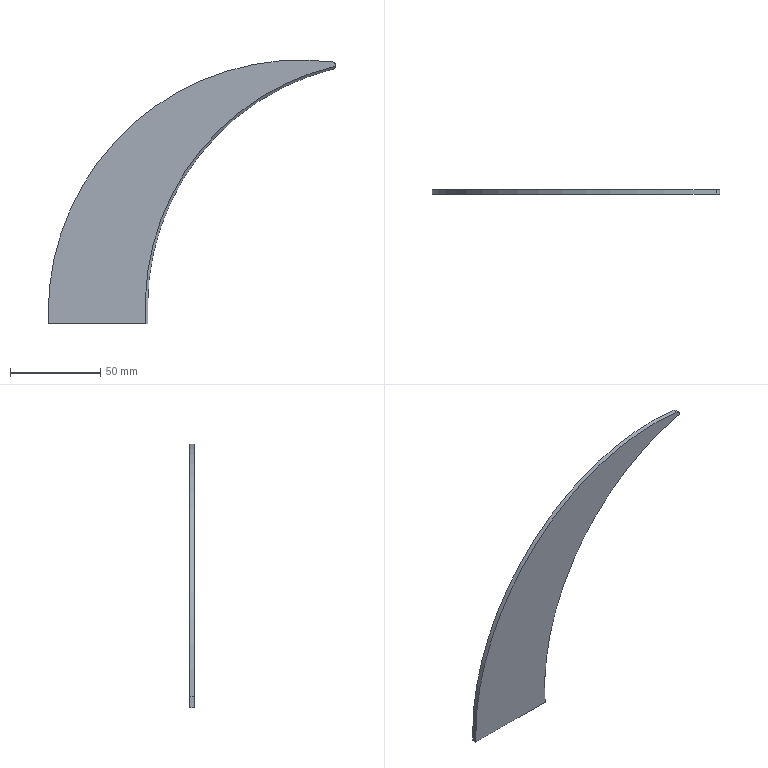Part | STEP file | DEWALT-DWE7492-B22 | 1 solid | 9 faces | box 159.2 x 2.5 x 146.092 mm | volume 19224 mm3 | plane 5 | cylinder 2 | cone 2 | commonest cylinder face diameters 4 x1 280 x1
STEP:
#1=CARTESIAN_POINT('',(0.,0.,0.));
#2=DIRECTION('',(0.,0.,1.));
#3=DIRECTION('',(1.,0.,0.));
#4=AXIS2_PLACEMENT_3D('',#1,#2,#3);
#5=CARTESIAN_POINT('',(54.117,2.5,0.));
#6=VERTEX_POINT('',#5);
#7=CARTESIAN_POINT('',(0.,2.5,0.));
#8=VERTEX_POINT('',#7);
#9=CARTESIAN_POINT('',(55.,2.5,0.));
#10=DIRECTION('',(-1.,0.,0.));
#11=VECTOR('',#10,1.);
#12=LINE('',#9,#11);
#13=CARTESIAN_POINT('',(55.,2.5,0.));
#14=DIRECTION('',(0.,0.,1.));
#15=DIRECTION('',(1.,0.,0.));
#16=AXIS2_PLACEMENT_3D('',#13,#14,#15);
#17=PLANE('',#16);
#18=CARTESIAN_POINT('',(0.,0.));
#19=DIRECTION('',(-1.,0.));
#20=VECTOR('',#19,1.);
#21=LINE('',#18,#20);
#22=(GEOMETRIC_REPRESENTATION_CONTEXT(2)PARAMETRIC_REPRESENTATION_CONTEXT()REPRESENTATION_CONTEXT('',''));
#23=DEFINITIONAL_REPRESENTATION('',(#21),#22);
#24=PCURVE('',#17,#23);
#25=CARTESIAN_POINT('',(140.,2.5,6.092));
#26=DIRECTION('',(0.,1.,0.));
#27=DIRECTION('',(0.,0.,1.));
#28=AXIS2_PLACEMENT_3D('',#25,#26,#27);
#29=PLANE('',#28);
#30=CARTESIAN_POINT('',(-6.092,-85.));
#31=DIRECTION('',(0.,-1.));
#32=VECTOR('',#31,1.);
#33=LINE('',#30,#32);
#34=(GEOMETRIC_REPRESENTATION_CONTEXT(2)PARAMETRIC_REPRESENTATION_CONTEXT()REPRESENTATION_CONTEXT('',''));
#35=DEFINITIONAL_REPRESENTATION('',(#33),#34);
#36=PCURVE('',#29,#35);
#37=SURFACE_CURVE('',#12,(#24,#36),.PCURVE_S1.);
#38=EDGE_CURVE('',#6,#8,#37,.T.);
#39=ORIENTED_EDGE('',*,*,#38,.F.);
#40=CARTESIAN_POINT('',(55.,1.62,0.));
#41=VERTEX_POINT('',#40);
#42=CARTESIAN_POINT('',(54.117,2.5,0.));
#43=CARTESIAN_POINT('',(54.412,2.207,0.));
#44=CARTESIAN_POINT('',(54.706,1.913,0.));
#45=CARTESIAN_POINT('',(55.,1.62,0.));
#46=B_SPLINE_CURVE_WITH_KNOTS('',3,(#42,#43,#44,#45),.UNSPECIFIED.,.F.,.F.,(4,4),(0.,0.001246),.PIECEWISE_BEZIER_KNOTS.);
#47=CARTESIAN_POINT('',(-0.8825,0.));
#48=CARTESIAN_POINT('',(-0.5884,-0.2934));
#49=CARTESIAN_POINT('',(-0.2942,-0.5868));
#50=CARTESIAN_POINT('',(0.,-0.8801));
#51=B_SPLINE_CURVE_WITH_KNOTS('',3,(#47,#48,#49,#50),.UNSPECIFIED.,.F.,.F.,(4,4),(0.,0.001246),.PIECEWISE_BEZIER_KNOTS.);
#52=(GEOMETRIC_REPRESENTATION_CONTEXT(2)PARAMETRIC_REPRESENTATION_CONTEXT()REPRESENTATION_CONTEXT('',''));
#53=DEFINITIONAL_REPRESENTATION('',(#51),#52);
#54=PCURVE('',#17,#53);
#55=CARTESIAN_POINT('',(190.,2.5,10.));
#56=DIRECTION('',(0.,1.,0.));
#57=DIRECTION('',(0.,0.,1.));
#58=AXIS2_PLACEMENT_3D('',#55,#56,#57);
#59=CONICAL_SURFACE('',#58,136.25,0.7854);
#60=CARTESIAN_POINT('',(4.639,0.));
#61=CARTESIAN_POINT('',(4.638,-0.8801));
#62=B_SPLINE_CURVE_WITH_KNOTS('',1,(#60,#61),.UNSPECIFIED.,.F.,.F.,(2,2),(0.,0.001246),.PIECEWISE_BEZIER_KNOTS.);
#63=(GEOMETRIC_REPRESENTATION_CONTEXT(2)PARAMETRIC_REPRESENTATION_CONTEXT()REPRESENTATION_CONTEXT('',''));
#64=DEFINITIONAL_REPRESENTATION('',(#62),#63);
#65=PCURVE('',#59,#64);
#66=SURFACE_CURVE('',#46,(#54,#65),.PCURVE_S1.);
#67=EDGE_CURVE('',#6,#41,#66,.T.);
#68=ORIENTED_EDGE('',*,*,#67,.T.);
#69=CARTESIAN_POINT('',(55.,0.8801,0.));
#70=VERTEX_POINT('',#69);
#71=CARTESIAN_POINT('',(55.,2.5,0.));
#72=DIRECTION('',(0.,-1.,0.));
#73=VECTOR('',#72,1.);
#74=LINE('',#71,#73);
#75=CARTESIAN_POINT('',(0.,0.));
#76=DIRECTION('',(0.,-1.));
#77=VECTOR('',#76,1.);
#78=LINE('',#75,#77);
#79=(GEOMETRIC_REPRESENTATION_CONTEXT(2)PARAMETRIC_REPRESENTATION_CONTEXT()REPRESENTATION_CONTEXT('',''));
#80=DEFINITIONAL_REPRESENTATION('',(#78),#79);
#81=PCURVE('',#17,#80);
#82=CARTESIAN_POINT('',(55.,2.5,10.));
#83=DIRECTION('',(-1.,0.,0.));
#84=DIRECTION('',(0.,0.,1.));
#85=AXIS2_PLACEMENT_3D('',#82,#83,#84);
#86=PLANE('',#85);
#87=CARTESIAN_POINT('',(-10.,0.));
#88=DIRECTION('',(0.,-1.));
#89=VECTOR('',#88,1.);
#90=LINE('',#87,#89);
#91=(GEOMETRIC_REPRESENTATION_CONTEXT(2)PARAMETRIC_REPRESENTATION_CONTEXT()REPRESENTATION_CONTEXT('',''));
#92=DEFINITIONAL_REPRESENTATION('',(#90),#91);
#93=PCURVE('',#86,#92);
#94=SURFACE_CURVE('',#74,(#81,#93),.PCURVE_S1.);
#95=EDGE_CURVE('',#41,#70,#94,.T.);
#96=ORIENTED_EDGE('',*,*,#95,.T.);
#97=CARTESIAN_POINT('',(54.117,0.,0.));
#98=VERTEX_POINT('',#97);
#99=CARTESIAN_POINT('',(55.,0.8801,0.));
#100=CARTESIAN_POINT('',(54.706,0.5868,0.));
#101=CARTESIAN_POINT('',(54.412,0.2934,0.));
#102=CARTESIAN_POINT('',(54.117,0.,0.));
#103=B_SPLINE_CURVE_WITH_KNOTS('',3,(#99,#100,#101,#102),.UNSPECIFIED.,.F.,.F.,(4,4),(0.,0.001246),.PIECEWISE_BEZIER_KNOTS.);
#104=CARTESIAN_POINT('',(0.,-1.62));
#105=CARTESIAN_POINT('',(-0.2942,-1.913));
#106=CARTESIAN_POINT('',(-0.5884,-2.207));
#107=CARTESIAN_POINT('',(-0.8825,-2.5));
#108=B_SPLINE_CURVE_WITH_KNOTS('',3,(#104,#105,#106,#107),.UNSPECIFIED.,.F.,.F.,(4,4),(0.,0.001246),.PIECEWISE_BEZIER_KNOTS.);
#109=(GEOMETRIC_REPRESENTATION_CONTEXT(2)PARAMETRIC_REPRESENTATION_CONTEXT()REPRESENTATION_CONTEXT('',''));
#110=DEFINITIONAL_REPRESENTATION('',(#108),#109);
#111=PCURVE('',#17,#110);
#112=CARTESIAN_POINT('',(190.,1.25,10.));
#113=DIRECTION('',(0.,-1.,0.));
#114=DIRECTION('',(0.,0.,-1.));
#115=AXIS2_PLACEMENT_3D('',#112,#113,#114);
#116=CONICAL_SURFACE('',#115,135.,0.7854);
#117=CARTESIAN_POINT('',(4.786,0.3699));
#118=CARTESIAN_POINT('',(4.786,1.25));
#119=B_SPLINE_CURVE_WITH_KNOTS('',1,(#117,#118),.UNSPECIFIED.,.F.,.F.,(2,2),(0.,0.001246),.PIECEWISE_BEZIER_KNOTS.);
#120=(GEOMETRIC_REPRESENTATION_CONTEXT(2)PARAMETRIC_REPRESENTATION_CONTEXT()REPRESENTATION_CONTEXT('',''));
#121=DEFINITIONAL_REPRESENTATION('',(#119),#120);
#122=PCURVE('',#116,#121);
#123=SURFACE_CURVE('',#103,(#111,#122),.PCURVE_S1.);
#124=EDGE_CURVE('',#70,#98,#123,.T.);
#125=ORIENTED_EDGE('',*,*,#124,.T.);
#126=CARTESIAN_POINT('',(0.,0.,0.));
#127=VERTEX_POINT('',#126);
#128=CARTESIAN_POINT('',(55.,0.,0.));
#129=DIRECTION('',(-1.,0.,0.));
#130=VECTOR('',#129,1.);
#131=LINE('',#128,#130);
#132=CARTESIAN_POINT('',(0.,-2.5));
#133=DIRECTION('',(-1.,0.));
#134=VECTOR('',#133,1.);
#135=LINE('',#132,#134);
#136=(GEOMETRIC_REPRESENTATION_CONTEXT(2)PARAMETRIC_REPRESENTATION_CONTEXT()REPRESENTATION_CONTEXT('',''));
#137=DEFINITIONAL_REPRESENTATION('',(#135),#136);
#138=PCURVE('',#17,#137);
#139=CARTESIAN_POINT('',(140.,0.,6.092));
#140=DIRECTION('',(0.,1.,0.));
#141=DIRECTION('',(0.,0.,1.));
#142=AXIS2_PLACEMENT_3D('',#139,#140,#141);
#143=PLANE('',#142);
#144=CARTESIAN_POINT('',(-6.092,-85.));
#145=DIRECTION('',(0.,-1.));
#146=VECTOR('',#145,1.);
#147=LINE('',#144,#146);
#148=(GEOMETRIC_REPRESENTATION_CONTEXT(2)PARAMETRIC_REPRESENTATION_CONTEXT()REPRESENTATION_CONTEXT('',''));
#149=DEFINITIONAL_REPRESENTATION('',(#147),#148);
#150=PCURVE('',#143,#149);
#151=SURFACE_CURVE('',#131,(#138,#150),.PCURVE_S1.);
#152=EDGE_CURVE('',#98,#127,#151,.T.);
#153=ORIENTED_EDGE('',*,*,#152,.T.);
#154=CARTESIAN_POINT('',(0.,2.5,0.));
#155=DIRECTION('',(0.,-1.,0.));
#156=VECTOR('',#155,1.);
#157=LINE('',#154,#156);
#158=CARTESIAN_POINT('',(-55.,0.));
#159=DIRECTION('',(0.,-1.));
#160=VECTOR('',#159,1.);
#161=LINE('',#158,#160);
#162=(GEOMETRIC_REPRESENTATION_CONTEXT(2)PARAMETRIC_REPRESENTATION_CONTEXT()REPRESENTATION_CONTEXT('',''));
#163=DEFINITIONAL_REPRESENTATION('',(#161),#162);
#164=PCURVE('',#17,#163);
#165=CARTESIAN_POINT('',(0.,2.5,0.));
#166=DIRECTION('',(1.,0.,0.));
#167=DIRECTION('',(0.,0.,-1.));
#168=AXIS2_PLACEMENT_3D('',#165,#166,#167);
#169=PLANE('',#168);
#170=CARTESIAN_POINT('',(0.,0.));
#171=DIRECTION('',(0.,-1.));
#172=VECTOR('',#171,1.);
#173=LINE('',#170,#172);
#174=(GEOMETRIC_REPRESENTATION_CONTEXT(2)PARAMETRIC_REPRESENTATION_CONTEXT()REPRESENTATION_CONTEXT('',''));
#175=DEFINITIONAL_REPRESENTATION('',(#173),#174);
#176=PCURVE('',#169,#175);
#177=SURFACE_CURVE('',#157,(#164,#176),.PCURVE_S1.);
#178=EDGE_CURVE('',#8,#127,#177,.T.);
#179=ORIENTED_EDGE('',*,*,#178,.F.);
#180=EDGE_LOOP('',(#39,#68,#96,#125,#153,#179));
#181=FACE_BOUND('',#180,.T.);
#182=ADVANCED_FACE('',(#181),#17,.F.);
#183=CARTESIAN_POINT('',(0.,0.,6.092));
#184=VERTEX_POINT('',#183);
#185=CARTESIAN_POINT('',(0.,0.,0.));
#186=DIRECTION('',(0.,0.,1.));
#187=VECTOR('',#186,1.);
#188=LINE('',#185,#187);
#189=CARTESIAN_POINT('',(0.,-2.5));
#190=DIRECTION('',(-1.,0.));
#191=VECTOR('',#190,1.);
#192=LINE('',#189,#191);
#193=(GEOMETRIC_REPRESENTATION_CONTEXT(2)PARAMETRIC_REPRESENTATION_CONTEXT()REPRESENTATION_CONTEXT('',''));
#194=DEFINITIONAL_REPRESENTATION('',(#192),#193);
#195=PCURVE('',#169,#194);
#196=CARTESIAN_POINT('',(-6.092,-140.));
#197=DIRECTION('',(1.,0.));
#198=VECTOR('',#197,1.);
#199=LINE('',#196,#198);
#200=(GEOMETRIC_REPRESENTATION_CONTEXT(2)PARAMETRIC_REPRESENTATION_CONTEXT()REPRESENTATION_CONTEXT('',''));
#201=DEFINITIONAL_REPRESENTATION('',(#199),#200);
#202=PCURVE('',#143,#201);
#203=SURFACE_CURVE('',#188,(#195,#202),.PCURVE_S1.);
#204=EDGE_CURVE('',#127,#184,#203,.T.);
#205=ORIENTED_EDGE('',*,*,#204,.T.);
#206=CARTESIAN_POINT('',(0.,2.5,6.092));
#207=VERTEX_POINT('',#206);
#208=CARTESIAN_POINT('',(0.,2.5,6.092));
#209=DIRECTION('',(0.,-1.,0.));
#210=VECTOR('',#209,1.);
#211=LINE('',#208,#210);
#212=CARTESIAN_POINT('',(-6.092,0.));
#213=DIRECTION('',(0.,-1.));
#214=VECTOR('',#213,1.);
#215=LINE('',#212,#214);
#216=(GEOMETRIC_REPRESENTATION_CONTEXT(2)PARAMETRIC_REPRESENTATION_CONTEXT()REPRESENTATION_CONTEXT('',''));
#217=DEFINITIONAL_REPRESENTATION('',(#215),#216);
#218=PCURVE('',#169,#217);
#219=CARTESIAN_POINT('',(140.,2.5,6.092));
#220=DIRECTION('',(0.,-1.,0.));
#221=DIRECTION('',(0.,0.,-1.));
#222=AXIS2_PLACEMENT_3D('',#219,#220,#221);
#223=CYLINDRICAL_SURFACE('',#222,140.);
#224=CARTESIAN_POINT('',(4.712,0.));
#225=DIRECTION('',(0.,1.));
#226=VECTOR('',#225,1.);
#227=LINE('',#224,#226);
#228=(GEOMETRIC_REPRESENTATION_CONTEXT(2)PARAMETRIC_REPRESENTATION_CONTEXT()REPRESENTATION_CONTEXT('',''));
#229=DEFINITIONAL_REPRESENTATION('',(#227),#228);
#230=PCURVE('',#223,#229);
#231=SURFACE_CURVE('',#211,(#218,#230),.PCURVE_S1.);
#232=EDGE_CURVE('',#207,#184,#231,.T.);
#233=ORIENTED_EDGE('',*,*,#232,.F.);
#234=CARTESIAN_POINT('',(0.,2.5,0.));
#235=DIRECTION('',(0.,0.,1.));
#236=VECTOR('',#235,1.);
#237=LINE('',#234,#236);
#238=CARTESIAN_POINT('',(0.,0.));
#239=DIRECTION('',(-1.,0.));
#240=VECTOR('',#239,1.);
#241=LINE('',#238,#240);
#242=(GEOMETRIC_REPRESENTATION_CONTEXT(2)PARAMETRIC_REPRESENTATION_CONTEXT()REPRESENTATION_CONTEXT('',''));
#243=DEFINITIONAL_REPRESENTATION('',(#241),#242);
#244=PCURVE('',#169,#243);
#245=CARTESIAN_POINT('',(-6.092,-140.));
#246=DIRECTION('',(1.,0.));
#247=VECTOR('',#246,1.);
#248=LINE('',#245,#247);
#249=(GEOMETRIC_REPRESENTATION_CONTEXT(2)PARAMETRIC_REPRESENTATION_CONTEXT()REPRESENTATION_CONTEXT('',''));
#250=DEFINITIONAL_REPRESENTATION('',(#248),#249);
#251=PCURVE('',#29,#250);
#252=SURFACE_CURVE('',#237,(#244,#251),.PCURVE_S1.);
#253=EDGE_CURVE('',#8,#207,#252,.T.);
#254=ORIENTED_EDGE('',*,*,#253,.F.);
#255=ORIENTED_EDGE('',*,*,#178,.T.);
#256=EDGE_LOOP('',(#205,#233,#254,#255));
#257=FACE_BOUND('',#256,.T.);
#258=ADVANCED_FACE('',(#257),#169,.F.);
#259=CARTESIAN_POINT('',(157.449,0.,145.));
#260=VERTEX_POINT('',#259);
#261=CARTESIAN_POINT('',(140.,0.,6.092));
#262=DIRECTION('',(0.,1.,0.));
#263=DIRECTION('',(1.,0.,0.));
#264=AXIS2_PLACEMENT_3D('',#261,#262,#263);
#265=CIRCLE('',#264,140.);
#266=CARTESIAN_POINT('',(7.854,2.5));
#267=DIRECTION('',(-1.,0.));
#268=VECTOR('',#267,1.);
#269=LINE('',#266,#268);
#270=(GEOMETRIC_REPRESENTATION_CONTEXT(2)PARAMETRIC_REPRESENTATION_CONTEXT()REPRESENTATION_CONTEXT('',''));
#271=DEFINITIONAL_REPRESENTATION('',(#269),#270);
#272=PCURVE('',#223,#271);
#273=CARTESIAN_POINT('',(0.,0.));
#274=DIRECTION('',(0.,1.));
#275=AXIS2_PLACEMENT_2D('',#273,#274);
#276=CIRCLE('',#275,140.);
#277=(GEOMETRIC_REPRESENTATION_CONTEXT(2)PARAMETRIC_REPRESENTATION_CONTEXT()REPRESENTATION_CONTEXT('',''));
#278=DEFINITIONAL_REPRESENTATION('',(#276),#277);
#279=PCURVE('',#143,#278);
#280=SURFACE_CURVE('',#265,(#272,#279),.PCURVE_S1.);
#281=EDGE_CURVE('',#184,#260,#280,.T.);
#282=ORIENTED_EDGE('',*,*,#281,.T.);
#283=CARTESIAN_POINT('',(157.449,2.5,145.));
#284=VERTEX_POINT('',#283);
#285=CARTESIAN_POINT('',(157.449,2.5,145.));
#286=DIRECTION('',(0.,-1.,0.));
#287=VECTOR('',#286,1.);
#288=LINE('',#285,#287);
#289=CARTESIAN_POINT('',(3.017,0.));
#290=DIRECTION('',(0.,1.));
#291=VECTOR('',#290,1.);
#292=LINE('',#289,#291);
#293=(GEOMETRIC_REPRESENTATION_CONTEXT(2)PARAMETRIC_REPRESENTATION_CONTEXT()REPRESENTATION_CONTEXT('',''));
#294=DEFINITIONAL_REPRESENTATION('',(#292),#293);
#295=PCURVE('',#223,#294);
#296=CARTESIAN_POINT('',(157.2,2.5,143.016));
#297=DIRECTION('',(0.,-1.,0.));
#298=DIRECTION('',(0.,0.,-1.));
#299=AXIS2_PLACEMENT_3D('',#296,#297,#298);
#300=CYLINDRICAL_SURFACE('',#299,2.);
#301=CARTESIAN_POINT('',(3.017,0.));
#302=DIRECTION('',(0.,1.));
#303=VECTOR('',#302,1.);
#304=LINE('',#301,#303);
#305=(GEOMETRIC_REPRESENTATION_CONTEXT(2)PARAMETRIC_REPRESENTATION_CONTEXT()REPRESENTATION_CONTEXT('',''));
#306=DEFINITIONAL_REPRESENTATION('',(#304),#305);
#307=PCURVE('',#300,#306);
#308=SURFACE_CURVE('',#288,(#295,#307),.PCURVE_S1.);
#309=EDGE_CURVE('',#284,#260,#308,.T.);
#310=ORIENTED_EDGE('',*,*,#309,.F.);
#311=CARTESIAN_POINT('',(140.,2.5,6.092));
#312=DIRECTION('',(0.,1.,0.));
#313=DIRECTION('',(1.,0.,0.));
#314=AXIS2_PLACEMENT_3D('',#311,#312,#313);
#315=CIRCLE('',#314,140.);
#316=CARTESIAN_POINT('',(7.854,0.));
#317=DIRECTION('',(-1.,0.));
#318=VECTOR('',#317,1.);
#319=LINE('',#316,#318);
#320=(GEOMETRIC_REPRESENTATION_CONTEXT(2)PARAMETRIC_REPRESENTATION_CONTEXT()REPRESENTATION_CONTEXT('',''));
#321=DEFINITIONAL_REPRESENTATION('',(#319),#320);
#322=PCURVE('',#223,#321);
#323=CARTESIAN_POINT('',(0.,0.));
#324=DIRECTION('',(0.,1.));
#325=AXIS2_PLACEMENT_2D('',#323,#324);
#326=CIRCLE('',#325,140.);
#327=(GEOMETRIC_REPRESENTATION_CONTEXT(2)PARAMETRIC_REPRESENTATION_CONTEXT()REPRESENTATION_CONTEXT('',''));
#328=DEFINITIONAL_REPRESENTATION('',(#326),#327);
#329=PCURVE('',#29,#328);
#330=SURFACE_CURVE('',#315,(#322,#329),.PCURVE_S1.);
#331=EDGE_CURVE('',#207,#284,#330,.T.);
#332=ORIENTED_EDGE('',*,*,#331,.F.);
#333=ORIENTED_EDGE('',*,*,#232,.T.);
#334=EDGE_LOOP('',(#282,#310,#332,#333));
#335=FACE_BOUND('',#334,.T.);
#336=ADVANCED_FACE('',(#335),#223,.T.);
#337=CARTESIAN_POINT('',(159.178,0.,142.718));
#338=VERTEX_POINT('',#337);
#339=CARTESIAN_POINT('',(157.679,1.25,141.074));
#340=VERTEX_POINT('',#339);
#341=CARTESIAN_POINT('',(159.178,0.,142.718));
#342=CARTESIAN_POINT('',(159.128,0.3116,142.386));
#343=CARTESIAN_POINT('',(158.872,0.9052,141.718));
#344=CARTESIAN_POINT('',(158.127,1.25,141.184));
#345=CARTESIAN_POINT('',(157.679,1.25,141.074));
#346=B_SPLINE_CURVE_WITH_KNOTS('',3,(#341,#342,#343,#344,#345),.UNSPECIFIED.,.F.,.F.,(4,1,4),(0.,0.001357,0.002714),.UNSPECIFIED.);
#347=CARTESIAN_POINT('',(1.421,2.5));
#348=CARTESIAN_POINT('',(1.406,2.472));
#349=CARTESIAN_POINT('',(1.376,2.415));
#350=CARTESIAN_POINT('',(1.329,2.332));
#351=CARTESIAN_POINT('',(1.283,2.249));
#352=CARTESIAN_POINT('',(1.236,2.168));
#353=CARTESIAN_POINT('',(1.188,2.088));
#354=CARTESIAN_POINT('',(1.14,2.011));
#355=CARTESIAN_POINT('',(1.091,1.935));
#356=CARTESIAN_POINT('',(1.041,1.861));
#357=CARTESIAN_POINT('',(0.991,1.79));
#358=CARTESIAN_POINT('',(0.9395,1.722));
#359=CARTESIAN_POINT('',(0.8869,1.656));
#360=CARTESIAN_POINT('',(0.8329,1.594));
#361=CARTESIAN_POINT('',(0.7777,1.535));
#362=CARTESIAN_POINT('',(0.7214,1.48));
#363=CARTESIAN_POINT('',(0.6641,1.43));
#364=CARTESIAN_POINT('',(0.606,1.385));
#365=CARTESIAN_POINT('',(0.5471,1.346));
#366=CARTESIAN_POINT('',(0.4875,1.312));
#367=CARTESIAN_POINT('',(0.4271,1.285));
#368=CARTESIAN_POINT('',(0.3661,1.265));
#369=CARTESIAN_POINT('',(0.3044,1.253));
#370=CARTESIAN_POINT('',(0.2627,1.25));
#371=CARTESIAN_POINT('',(0.2418,1.25));
#372=B_SPLINE_CURVE_WITH_KNOTS('',3,(#347,#348,#349,#350,#351,#352,#353,#354,#355,#356,#357,#358,#359,#360,#361,#362,#363,#364,#365,#366,#367,#368,#369,#370,#371),.UNSPECIFIED.,.F.,.F.,(4,1,1,1,1,1,1,1,1,1,1,1,1,1,1,1,1,1,1,1,1,1,4),(0.,0.0001234,0.0002467,0.0003701,0.0004934,0.0006168,0.0007401,0.0008635,0.0009868,0.00111,0.001234,0.001357,0.00148,0.001604,0.001727,0.00185,0.001974,0.002097,0.00222,0.002344,0.002467,0.00259,0.002714),.QUASI_UNIFORM_KNOTS.);
#373=(GEOMETRIC_REPRESENTATION_CONTEXT(2)PARAMETRIC_REPRESENTATION_CONTEXT()REPRESENTATION_CONTEXT('',''));
#374=DEFINITIONAL_REPRESENTATION('',(#372),#373);
#375=PCURVE('',#300,#374);
#376=CARTESIAN_POINT('',(3.37,1.25));
#377=CARTESIAN_POINT('',(3.37,1.222));
#378=CARTESIAN_POINT('',(3.37,1.165));
#379=CARTESIAN_POINT('',(3.37,1.082));
#380=CARTESIAN_POINT('',(3.371,0.9991));
#381=CARTESIAN_POINT('',(3.371,0.918));
#382=CARTESIAN_POINT('',(3.371,0.8384));
#383=CARTESIAN_POINT('',(3.372,0.7607));
#384=CARTESIAN_POINT('',(3.372,0.685));
#385=CARTESIAN_POINT('',(3.373,0.6115));
#386=CARTESIAN_POINT('',(3.373,0.5404));
#387=CARTESIAN_POINT('',(3.374,0.472));
#388=CARTESIAN_POINT('',(3.374,0.4065));
#389=CARTESIAN_POINT('',(3.375,0.344));
#390=CARTESIAN_POINT('',(3.376,0.2852));
#391=CARTESIAN_POINT('',(3.377,0.2304));
#392=CARTESIAN_POINT('',(3.377,0.1802));
#393=CARTESIAN_POINT('',(3.378,0.135));
#394=CARTESIAN_POINT('',(3.379,0.09548));
#395=CARTESIAN_POINT('',(3.38,0.06198));
#396=CARTESIAN_POINT('',(3.381,0.03504));
#397=CARTESIAN_POINT('',(3.382,0.01517));
#398=CARTESIAN_POINT('',(3.382,0.002848));
#399=CARTESIAN_POINT('',(3.383,-0.000000049));
#400=CARTESIAN_POINT('',(3.383,0.));
#401=B_SPLINE_CURVE_WITH_KNOTS('',3,(#376,#377,#378,#379,#380,#381,#382,#383,#384,#385,#386,#387,#388,#389,#390,#391,#392,#393,#394,#395,#396,#397,#398,#399,#400),.UNSPECIFIED.,.F.,.F.,(4,1,1,1,1,1,1,1,1,1,1,1,1,1,1,1,1,1,1,1,1,1,4),(0.,0.0001234,0.0002467,0.0003701,0.0004934,0.0006168,0.0007401,0.0008635,0.0009868,0.00111,0.001234,0.001357,0.00148,0.001604,0.001727,0.00185,0.001974,0.002097,0.00222,0.002344,0.002467,0.00259,0.002714),.QUASI_UNIFORM_KNOTS.);
#402=(GEOMETRIC_REPRESENTATION_CONTEXT(2)PARAMETRIC_REPRESENTATION_CONTEXT()REPRESENTATION_CONTEXT('',''));
#403=DEFINITIONAL_REPRESENTATION('',(#401),#402);
#404=PCURVE('',#116,#403);
#405=SURFACE_CURVE('',#346,(#375,#404),.PCURVE_S1.);
#406=EDGE_CURVE('',#338,#340,#405,.T.);
#407=ORIENTED_EDGE('',*,*,#406,.T.);
#408=CARTESIAN_POINT('',(159.178,2.5,142.718));
#409=VERTEX_POINT('',#408);
#410=CARTESIAN_POINT('',(157.679,1.25,141.074));
#411=CARTESIAN_POINT('',(158.127,1.25,141.184));
#412=CARTESIAN_POINT('',(158.871,1.594,141.717));
#413=CARTESIAN_POINT('',(159.128,2.188,142.386));
#414=CARTESIAN_POINT('',(159.178,2.5,142.718));
#415=B_SPLINE_CURVE_WITH_KNOTS('',3,(#410,#411,#412,#413,#414),.UNSPECIFIED.,.F.,.F.,(4,1,4),(0.,0.00136,0.002721),.UNSPECIFIED.);
#416=CARTESIAN_POINT('',(0.2418,1.25));
#417=CARTESIAN_POINT('',(0.2627,1.25));
#418=CARTESIAN_POINT('',(0.3044,1.247));
#419=CARTESIAN_POINT('',(0.3661,1.235));
#420=CARTESIAN_POINT('',(0.4271,1.215));
#421=CARTESIAN_POINT('',(0.4873,1.188));
#422=CARTESIAN_POINT('',(0.5469,1.155));
#423=CARTESIAN_POINT('',(0.6058,1.115));
#424=CARTESIAN_POINT('',(0.6639,1.07));
#425=CARTESIAN_POINT('',(0.7211,1.02));
#426=CARTESIAN_POINT('',(0.7773,0.9653));
#427=CARTESIAN_POINT('',(0.8325,0.9064));
#428=CARTESIAN_POINT('',(0.8865,0.844));
#429=CARTESIAN_POINT('',(0.9391,0.7785));
#430=CARTESIAN_POINT('',(0.9906,0.7101));
#431=CARTESIAN_POINT('',(1.041,0.639));
#432=CARTESIAN_POINT('',(1.091,0.5654));
#433=CARTESIAN_POINT('',(1.14,0.4896));
#434=CARTESIAN_POINT('',(1.188,0.4118));
#435=CARTESIAN_POINT('',(1.235,0.3322));
#436=CARTESIAN_POINT('',(1.283,0.251));
#437=CARTESIAN_POINT('',(1.329,0.1685));
#438=CARTESIAN_POINT('',(1.376,0.08477));
#439=CARTESIAN_POINT('',(1.406,0.02834));
#440=CARTESIAN_POINT('',(1.421,0.));
#441=B_SPLINE_CURVE_WITH_KNOTS('',3,(#416,#417,#418,#419,#420,#421,#422,#423,#424,#425,#426,#427,#428,#429,#430,#431,#432,#433,#434,#435,#436,#437,#438,#439,#440),.UNSPECIFIED.,.F.,.F.,(4,1,1,1,1,1,1,1,1,1,1,1,1,1,1,1,1,1,1,1,1,1,4),(0.,0.0001237,0.0002473,0.000371,0.0004947,0.0006183,0.000742,0.0008657,0.0009893,0.001113,0.001237,0.00136,0.001484,0.001608,0.001731,0.001855,0.001979,0.002102,0.002226,0.00235,0.002473,0.002597,0.002721),.QUASI_UNIFORM_KNOTS.);
#442=(GEOMETRIC_REPRESENTATION_CONTEXT(2)PARAMETRIC_REPRESENTATION_CONTEXT()REPRESENTATION_CONTEXT('',''));
#443=DEFINITIONAL_REPRESENTATION('',(#441),#442);
#444=PCURVE('',#300,#443);
#445=CARTESIAN_POINT('',(6.041,-1.25));
#446=CARTESIAN_POINT('',(6.042,-1.25));
#447=CARTESIAN_POINT('',(6.042,-1.247));
#448=CARTESIAN_POINT('',(6.043,-1.235));
#449=CARTESIAN_POINT('',(6.044,-1.215));
#450=CARTESIAN_POINT('',(6.045,-1.188));
#451=CARTESIAN_POINT('',(6.046,-1.155));
#452=CARTESIAN_POINT('',(6.047,-1.115));
#453=CARTESIAN_POINT('',(6.047,-1.07));
#454=CARTESIAN_POINT('',(6.048,-1.02));
#455=CARTESIAN_POINT('',(6.049,-0.9653));
#456=CARTESIAN_POINT('',(6.05,-0.9064));
#457=CARTESIAN_POINT('',(6.05,-0.844));
#458=CARTESIAN_POINT('',(6.051,-0.7785));
#459=CARTESIAN_POINT('',(6.051,-0.71));
#460=CARTESIAN_POINT('',(6.052,-0.6389));
#461=CARTESIAN_POINT('',(6.053,-0.5654));
#462=CARTESIAN_POINT('',(6.053,-0.4896));
#463=CARTESIAN_POINT('',(6.053,-0.4118));
#464=CARTESIAN_POINT('',(6.054,-0.3322));
#465=CARTESIAN_POINT('',(6.054,-0.251));
#466=CARTESIAN_POINT('',(6.054,-0.1685));
#467=CARTESIAN_POINT('',(6.055,-0.08477));
#468=CARTESIAN_POINT('',(6.055,-0.02834));
#469=CARTESIAN_POINT('',(6.055,0.));
#470=B_SPLINE_CURVE_WITH_KNOTS('',3,(#445,#446,#447,#448,#449,#450,#451,#452,#453,#454,#455,#456,#457,#458,#459,#460,#461,#462,#463,#464,#465,#466,#467,#468,#469),.UNSPECIFIED.,.F.,.F.,(4,1,1,1,1,1,1,1,1,1,1,1,1,1,1,1,1,1,1,1,1,1,4),(0.,0.0001237,0.0002473,0.000371,0.0004947,0.0006183,0.000742,0.0008657,0.0009893,0.001113,0.001237,0.00136,0.001484,0.001608,0.001731,0.001855,0.001979,0.002102,0.002226,0.00235,0.002473,0.002597,0.002721),.QUASI_UNIFORM_KNOTS.);
#471=(GEOMETRIC_REPRESENTATION_CONTEXT(2)PARAMETRIC_REPRESENTATION_CONTEXT()REPRESENTATION_CONTEXT('',''));
#472=DEFINITIONAL_REPRESENTATION('',(#470),#471);
#473=PCURVE('',#59,#472);
#474=SURFACE_CURVE('',#415,(#444,#473),.PCURVE_S1.);
#475=EDGE_CURVE('',#340,#409,#474,.T.);
#476=ORIENTED_EDGE('',*,*,#475,.T.);
#477=CARTESIAN_POINT('',(157.2,2.5,143.016));
#478=DIRECTION('',(0.,1.,0.));
#479=DIRECTION('',(-1.,0.,0.));
#480=AXIS2_PLACEMENT_3D('',#477,#478,#479);
#481=CIRCLE('',#480,2.);
#482=CARTESIAN_POINT('',(4.712,0.));
#483=DIRECTION('',(-1.,0.));
#484=VECTOR('',#483,1.);
#485=LINE('',#482,#484);
#486=(GEOMETRIC_REPRESENTATION_CONTEXT(2)PARAMETRIC_REPRESENTATION_CONTEXT()REPRESENTATION_CONTEXT('',''));
#487=DEFINITIONAL_REPRESENTATION('',(#485),#486);
#488=PCURVE('',#300,#487);
#489=CARTESIAN_POINT('',(136.924,17.2));
#490=DIRECTION('',(0.,-1.));
#491=AXIS2_PLACEMENT_2D('',#489,#490);
#492=CIRCLE('',#491,2.);
#493=(GEOMETRIC_REPRESENTATION_CONTEXT(2)PARAMETRIC_REPRESENTATION_CONTEXT()REPRESENTATION_CONTEXT('',''));
#494=DEFINITIONAL_REPRESENTATION('',(#492),#493);
#495=PCURVE('',#29,#494);
#496=SURFACE_CURVE('',#481,(#488,#495),.PCURVE_S1.);
#497=EDGE_CURVE('',#284,#409,#496,.T.);
#498=ORIENTED_EDGE('',*,*,#497,.F.);
#499=ORIENTED_EDGE('',*,*,#309,.T.);
#500=CARTESIAN_POINT('',(157.2,0.,143.016));
#501=DIRECTION('',(0.,1.,0.));
#502=DIRECTION('',(-1.,0.,0.));
#503=AXIS2_PLACEMENT_3D('',#500,#501,#502);
#504=CIRCLE('',#503,2.);
#505=CARTESIAN_POINT('',(4.712,2.5));
#506=DIRECTION('',(-1.,0.));
#507=VECTOR('',#506,1.);
#508=LINE('',#505,#507);
#509=(GEOMETRIC_REPRESENTATION_CONTEXT(2)PARAMETRIC_REPRESENTATION_CONTEXT()REPRESENTATION_CONTEXT('',''));
#510=DEFINITIONAL_REPRESENTATION('',(#508),#509);
#511=PCURVE('',#300,#510);
#512=CARTESIAN_POINT('',(136.924,17.2));
#513=DIRECTION('',(0.,-1.));
#514=AXIS2_PLACEMENT_2D('',#512,#513);
#515=CIRCLE('',#514,2.);
#516=(GEOMETRIC_REPRESENTATION_CONTEXT(2)PARAMETRIC_REPRESENTATION_CONTEXT()REPRESENTATION_CONTEXT('',''));
#517=DEFINITIONAL_REPRESENTATION('',(#515),#516);
#518=PCURVE('',#143,#517);
#519=SURFACE_CURVE('',#504,(#511,#518),.PCURVE_S1.);
#520=EDGE_CURVE('',#260,#338,#519,.T.);
#521=ORIENTED_EDGE('',*,*,#520,.T.);
#522=EDGE_LOOP('',(#407,#476,#498,#499,#521));
#523=FACE_BOUND('',#522,.T.);
#524=ADVANCED_FACE('',(#523),#300,.T.);
#525=ORIENTED_EDGE('',*,*,#95,.F.);
#526=CARTESIAN_POINT('',(55.,1.25,10.));
#527=VERTEX_POINT('',#526);
#528=CARTESIAN_POINT('',(55.,1.62,0.));
#529=CARTESIAN_POINT('',(55.,1.374,3.329));
#530=CARTESIAN_POINT('',(55.,1.25,6.662));
#531=CARTESIAN_POINT('',(55.,1.25,10.));
#532=B_SPLINE_CURVE_WITH_KNOTS('',3,(#528,#529,#530,#531),.UNSPECIFIED.,.F.,.F.,(4,4),(0.,0.01001),.PIECEWISE_BEZIER_KNOTS.);
#533=CARTESIAN_POINT('',(-10.,-0.8801));
#534=CARTESIAN_POINT('',(-6.671,-1.126));
#535=CARTESIAN_POINT('',(-3.338,-1.25));
#536=CARTESIAN_POINT('',(0.,-1.25));
#537=B_SPLINE_CURVE_WITH_KNOTS('',3,(#533,#534,#535,#536),.UNSPECIFIED.,.F.,.F.,(4,4),(0.,0.01001),.PIECEWISE_BEZIER_KNOTS.);
#538=(GEOMETRIC_REPRESENTATION_CONTEXT(2)PARAMETRIC_REPRESENTATION_CONTEXT()REPRESENTATION_CONTEXT('',''));
#539=DEFINITIONAL_REPRESENTATION('',(#537),#538);
#540=PCURVE('',#86,#539);
#541=CARTESIAN_POINT('',(4.638,-0.8801));
#542=CARTESIAN_POINT('',(4.64,-0.8913));
#543=CARTESIAN_POINT('',(4.642,-0.9132));
#544=CARTESIAN_POINT('',(4.645,-0.9444));
#545=CARTESIAN_POINT('',(4.648,-0.9742));
#546=CARTESIAN_POINT('',(4.652,-1.002));
#547=CARTESIAN_POINT('',(4.655,-1.029));
#548=CARTESIAN_POINT('',(4.659,-1.054));
#549=CARTESIAN_POINT('',(4.662,-1.078));
#550=CARTESIAN_POINT('',(4.665,-1.1));
#551=CARTESIAN_POINT('',(4.669,-1.121));
#552=CARTESIAN_POINT('',(4.672,-1.14));
#553=CARTESIAN_POINT('',(4.675,-1.158));
#554=CARTESIAN_POINT('',(4.679,-1.174));
#555=CARTESIAN_POINT('',(4.682,-1.188));
#556=CARTESIAN_POINT('',(4.685,-1.201));
#557=CARTESIAN_POINT('',(4.689,-1.213));
#558=CARTESIAN_POINT('',(4.692,-1.223));
#559=CARTESIAN_POINT('',(4.696,-1.231));
#560=CARTESIAN_POINT('',(4.699,-1.238));
#561=CARTESIAN_POINT('',(4.702,-1.243));
#562=CARTESIAN_POINT('',(4.706,-1.247));
#563=CARTESIAN_POINT('',(4.709,-1.249));
#564=CARTESIAN_POINT('',(4.711,-1.25));
#565=CARTESIAN_POINT('',(4.712,-1.25));
#566=B_SPLINE_CURVE_WITH_KNOTS('',3,(#541,#542,#543,#544,#545,#546,#547,#548,#549,#550,#551,#552,#553,#554,#555,#556,#557,#558,#559,#560,#561,#562,#563,#564,#565),.UNSPECIFIED.,.F.,.F.,(4,1,1,1,1,1,1,1,1,1,1,1,1,1,1,1,1,1,1,1,1,1,4),(0.,0.0004549,0.0009097,0.001365,0.001819,0.002274,0.002729,0.003184,0.003639,0.004094,0.004549,0.005003,0.005458,0.005913,0.006368,0.006823,0.007278,0.007733,0.008187,0.008642,0.009097,0.009552,0.01001),.QUASI_UNIFORM_KNOTS.);
#567=(GEOMETRIC_REPRESENTATION_CONTEXT(2)PARAMETRIC_REPRESENTATION_CONTEXT()REPRESENTATION_CONTEXT('',''));
#568=DEFINITIONAL_REPRESENTATION('',(#566),#567);
#569=PCURVE('',#59,#568);
#570=SURFACE_CURVE('',#532,(#540,#569),.PCURVE_S1.);
#571=EDGE_CURVE('',#41,#527,#570,.T.);
#572=ORIENTED_EDGE('',*,*,#571,.T.);
#573=CARTESIAN_POINT('',(55.,1.25,10.));
#574=CARTESIAN_POINT('',(55.,1.25,6.662));
#575=CARTESIAN_POINT('',(55.,1.126,3.329));
#576=CARTESIAN_POINT('',(55.,0.8801,0.));
#577=B_SPLINE_CURVE_WITH_KNOTS('',3,(#573,#574,#575,#576),.UNSPECIFIED.,.F.,.F.,(4,4),(0.,0.01001),.PIECEWISE_BEZIER_KNOTS.);
#578=CARTESIAN_POINT('',(0.,-1.25));
#579=CARTESIAN_POINT('',(-3.338,-1.25));
#580=CARTESIAN_POINT('',(-6.671,-1.374));
#581=CARTESIAN_POINT('',(-10.,-1.62));
#582=B_SPLINE_CURVE_WITH_KNOTS('',3,(#578,#579,#580,#581),.UNSPECIFIED.,.F.,.F.,(4,4),(0.,0.01001),.PIECEWISE_BEZIER_KNOTS.);
#583=(GEOMETRIC_REPRESENTATION_CONTEXT(2)PARAMETRIC_REPRESENTATION_CONTEXT()REPRESENTATION_CONTEXT('',''));
#584=DEFINITIONAL_REPRESENTATION('',(#582),#583);
#585=PCURVE('',#86,#584);
#586=CARTESIAN_POINT('',(4.712,0.));
#587=CARTESIAN_POINT('',(4.714,-0.000000002));
#588=CARTESIAN_POINT('',(4.716,0.0005119));
#589=CARTESIAN_POINT('',(4.719,0.002815));
#590=CARTESIAN_POINT('',(4.723,0.006651));
#591=CARTESIAN_POINT('',(4.726,0.01202));
#592=CARTESIAN_POINT('',(4.729,0.01892));
#593=CARTESIAN_POINT('',(4.733,0.02735));
#594=CARTESIAN_POINT('',(4.736,0.03732));
#595=CARTESIAN_POINT('',(4.739,0.04881));
#596=CARTESIAN_POINT('',(4.743,0.06183));
#597=CARTESIAN_POINT('',(4.746,0.07638));
#598=CARTESIAN_POINT('',(4.749,0.09245));
#599=CARTESIAN_POINT('',(4.753,0.11));
#600=CARTESIAN_POINT('',(4.756,0.1292));
#601=CARTESIAN_POINT('',(4.76,0.1498));
#602=CARTESIAN_POINT('',(4.763,0.172));
#603=CARTESIAN_POINT('',(4.766,0.1957));
#604=CARTESIAN_POINT('',(4.77,0.2209));
#605=CARTESIAN_POINT('',(4.773,0.2476));
#606=CARTESIAN_POINT('',(4.776,0.2758));
#607=CARTESIAN_POINT('',(4.78,0.3056));
#608=CARTESIAN_POINT('',(4.783,0.3368));
#609=CARTESIAN_POINT('',(4.785,0.3587));
#610=CARTESIAN_POINT('',(4.786,0.3699));
#611=B_SPLINE_CURVE_WITH_KNOTS('',3,(#586,#587,#588,#589,#590,#591,#592,#593,#594,#595,#596,#597,#598,#599,#600,#601,#602,#603,#604,#605,#606,#607,#608,#609,#610),.UNSPECIFIED.,.F.,.F.,(4,1,1,1,1,1,1,1,1,1,1,1,1,1,1,1,1,1,1,1,1,1,4),(0.,0.0004549,0.0009097,0.001365,0.001819,0.002274,0.002729,0.003184,0.003639,0.004094,0.004549,0.005003,0.005458,0.005913,0.006368,0.006823,0.007278,0.007733,0.008187,0.008642,0.009097,0.009552,0.01001),.QUASI_UNIFORM_KNOTS.);
#612=(GEOMETRIC_REPRESENTATION_CONTEXT(2)PARAMETRIC_REPRESENTATION_CONTEXT()REPRESENTATION_CONTEXT('',''));
#613=DEFINITIONAL_REPRESENTATION('',(#611),#612);
#614=PCURVE('',#116,#613);
#615=SURFACE_CURVE('',#577,(#585,#614),.PCURVE_S1.);
#616=EDGE_CURVE('',#527,#70,#615,.T.);
#617=ORIENTED_EDGE('',*,*,#616,.T.);
#618=EDGE_LOOP('',(#525,#572,#617));
#619=FACE_BOUND('',#618,.T.);
#620=ADVANCED_FACE('',(#619),#86,.F.);
#621=ORIENTED_EDGE('',*,*,#497,.T.);
#622=CARTESIAN_POINT('',(190.,2.5,10.));
#623=DIRECTION('',(0.,1.,0.));
#624=DIRECTION('',(0.,0.,1.));
#625=AXIS2_PLACEMENT_3D('',#622,#623,#624);
#626=CIRCLE('',#625,136.25);
#627=CARTESIAN_POINT('',(3.908,50.));
#628=DIRECTION('',(1.,0.));
#629=AXIS2_PLACEMENT_2D('',#627,#628);
#630=CIRCLE('',#629,136.25);
#631=(GEOMETRIC_REPRESENTATION_CONTEXT(2)PARAMETRIC_REPRESENTATION_CONTEXT()REPRESENTATION_CONTEXT('',''));
#632=DEFINITIONAL_REPRESENTATION('',(#630),#631);
#633=PCURVE('',#29,#632);
#634=CARTESIAN_POINT('',(0.,0.));
#635=DIRECTION('',(1.,0.));
#636=VECTOR('',#635,1.);
#637=LINE('',#634,#636);
#638=(GEOMETRIC_REPRESENTATION_CONTEXT(2)PARAMETRIC_REPRESENTATION_CONTEXT()REPRESENTATION_CONTEXT('',''));
#639=DEFINITIONAL_REPRESENTATION('',(#637),#638);
#640=PCURVE('',#59,#639);
#641=SURFACE_CURVE('',#626,(#633,#640),.PCURVE_S1.);
#642=EDGE_CURVE('',#6,#409,#641,.T.);
#643=ORIENTED_EDGE('',*,*,#642,.F.);
#644=ORIENTED_EDGE('',*,*,#38,.T.);
#645=ORIENTED_EDGE('',*,*,#253,.T.);
#646=ORIENTED_EDGE('',*,*,#331,.T.);
#647=EDGE_LOOP('',(#621,#643,#644,#645,#646));
#648=FACE_BOUND('',#647,.T.);
#649=ADVANCED_FACE('',(#648),#29,.T.);
#650=ORIENTED_EDGE('',*,*,#152,.F.);
#651=CARTESIAN_POINT('',(190.,0.,10.));
#652=DIRECTION('',(0.,1.,0.));
#653=DIRECTION('',(0.,0.,1.));
#654=AXIS2_PLACEMENT_3D('',#651,#652,#653);
#655=CIRCLE('',#654,136.25);
#656=CARTESIAN_POINT('',(3.908,50.));
#657=DIRECTION('',(1.,0.));
#658=AXIS2_PLACEMENT_2D('',#656,#657);
#659=CIRCLE('',#658,136.25);
#660=(GEOMETRIC_REPRESENTATION_CONTEXT(2)PARAMETRIC_REPRESENTATION_CONTEXT()REPRESENTATION_CONTEXT('',''));
#661=DEFINITIONAL_REPRESENTATION('',(#659),#660);
#662=PCURVE('',#143,#661);
#663=CARTESIAN_POINT('',(9.425,1.25));
#664=DIRECTION('',(-1.,0.));
#665=VECTOR('',#664,1.);
#666=LINE('',#663,#665);
#667=(GEOMETRIC_REPRESENTATION_CONTEXT(2)PARAMETRIC_REPRESENTATION_CONTEXT()REPRESENTATION_CONTEXT('',''));
#668=DEFINITIONAL_REPRESENTATION('',(#666),#667);
#669=PCURVE('',#116,#668);
#670=SURFACE_CURVE('',#655,(#662,#669),.PCURVE_S1.);
#671=EDGE_CURVE('',#98,#338,#670,.T.);
#672=ORIENTED_EDGE('',*,*,#671,.T.);
#673=ORIENTED_EDGE('',*,*,#520,.F.);
#674=ORIENTED_EDGE('',*,*,#281,.F.);
#675=ORIENTED_EDGE('',*,*,#204,.F.);
#676=EDGE_LOOP('',(#650,#672,#673,#674,#675));
#677=FACE_BOUND('',#676,.T.);
#678=ADVANCED_FACE('',(#677),#143,.F.);
#679=CARTESIAN_POINT('',(190.,1.25,10.));
#680=DIRECTION('',(0.,1.,0.));
#681=DIRECTION('',(0.,0.,1.));
#682=AXIS2_PLACEMENT_3D('',#679,#680,#681);
#683=CIRCLE('',#682,135.);
#684=CARTESIAN_POINT('',(9.425,0.));
#685=DIRECTION('',(-1.,0.));
#686=VECTOR('',#685,1.);
#687=LINE('',#684,#686);
#688=(GEOMETRIC_REPRESENTATION_CONTEXT(2)PARAMETRIC_REPRESENTATION_CONTEXT()REPRESENTATION_CONTEXT('',''));
#689=DEFINITIONAL_REPRESENTATION('',(#687),#688);
#690=PCURVE('',#116,#689);
#691=CARTESIAN_POINT('',(0.,-1.25));
#692=DIRECTION('',(1.,0.));
#693=VECTOR('',#692,1.);
#694=LINE('',#691,#693);
#695=(GEOMETRIC_REPRESENTATION_CONTEXT(2)PARAMETRIC_REPRESENTATION_CONTEXT()REPRESENTATION_CONTEXT('',''));
#696=DEFINITIONAL_REPRESENTATION('',(#694),#695);
#697=PCURVE('',#59,#696);
#698=SURFACE_CURVE('',#683,(#690,#697),.PCURVE_S1.);
#699=EDGE_CURVE('',#527,#340,#698,.T.);
#700=ORIENTED_EDGE('',*,*,#699,.F.);
#701=ORIENTED_EDGE('',*,*,#616,.T.);
#702=ORIENTED_EDGE('',*,*,#124,.T.);
#703=ORIENTED_EDGE('',*,*,#671,.T.);
#704=ORIENTED_EDGE('',*,*,#406,.T.);
#705=EDGE_LOOP('',(#700,#701,#702,#703,#704));
#706=FACE_BOUND('',#705,.F.);
#707=ADVANCED_FACE('',(#706),#116,.F.);
#708=ORIENTED_EDGE('',*,*,#642,.F.);
#709=ORIENTED_EDGE('',*,*,#67,.T.);
#710=ORIENTED_EDGE('',*,*,#571,.T.);
#711=ORIENTED_EDGE('',*,*,#699,.T.);
#712=ORIENTED_EDGE('',*,*,#475,.T.);
#713=EDGE_LOOP('',(#708,#709,#710,#711,#712));
#714=FACE_BOUND('',#713,.F.);
#715=ADVANCED_FACE('',(#714),#59,.F.);
#716=CLOSED_SHELL('',(#182,#258,#336,#524,#620,#649,#678,#707,#715));
#717=MANIFOLD_SOLID_BREP('',#716);
#718=(LENGTH_UNIT()NAMED_UNIT(*)SI_UNIT(.MILLI.,.METRE.));
#719=UNCERTAINTY_MEASURE_WITH_UNIT(LENGTH_MEASURE(0.0005),#718,'','');
#720=(NAMED_UNIT(*)PLANE_ANGLE_UNIT()SI_UNIT($,.RADIAN.));
#721=(NAMED_UNIT(*)SI_UNIT($,.STERADIAN.)SOLID_ANGLE_UNIT());
#722=(GEOMETRIC_REPRESENTATION_CONTEXT(3)GLOBAL_UNCERTAINTY_ASSIGNED_CONTEXT((#719))GLOBAL_UNIT_ASSIGNED_CONTEXT((#718,#720,#721))REPRESENTATION_CONTEXT('',''));
#723=ADVANCED_BREP_SHAPE_REPRESENTATION('',(#4,#717),#722);